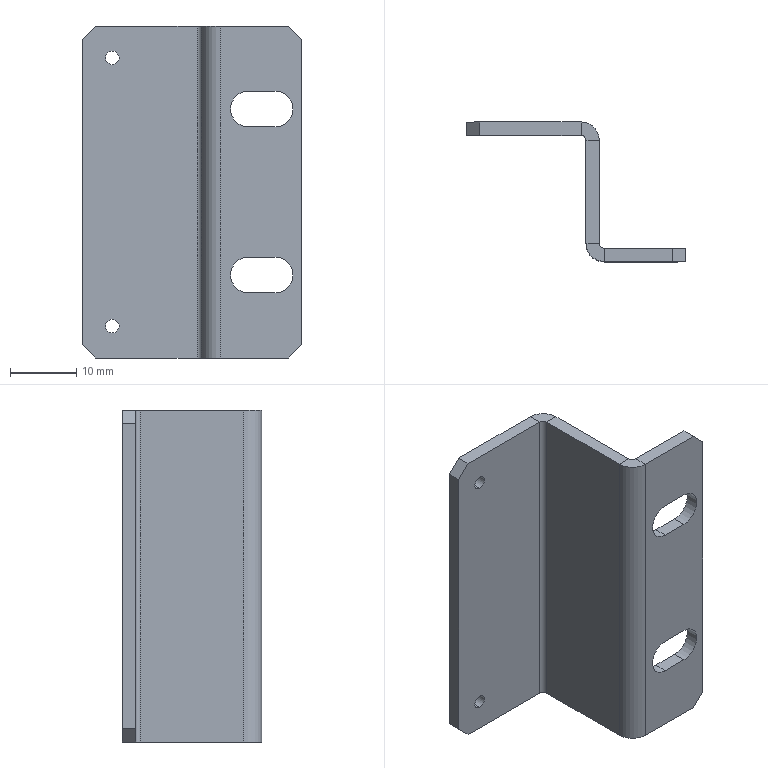Part | STEP file | 11-GYZB-JJ-00611 | 1 solid | 38 faces | box 33 x 21 x 50 mm | volume 4844 mm3 | plane 26 | cylinder 12 | commonest cylinder face diameters 2.05 x4 5.4 x4 1.473 x2 5.473 x2
STEP:
#1=CARTESIAN_POINT('',(-13.5,19.,-21.225));
#2=VERTEX_POINT('',#1);
#3=CARTESIAN_POINT('',(-13.5,19.,-19.175));
#4=VERTEX_POINT('',#3);
#5=CARTESIAN_POINT('',(-13.5,19.,-20.2));
#6=DIRECTION('',(0.,1.,0.));
#7=DIRECTION('',(-1.,0.,0.));
#8=AXIS2_PLACEMENT_3D('',#5,#6,#7);
#9=CIRCLE('',#8,1.025);
#10=EDGE_CURVE('',#2,#4,#9,.T.);
#11=ORIENTED_EDGE('',*,*,#10,.F.);
#12=CARTESIAN_POINT('',(-13.5,21.,-21.225));
#13=VERTEX_POINT('',#12);
#14=CARTESIAN_POINT('',(-13.5,21.,-21.225));
#15=DIRECTION('',(0.,1.,0.));
#16=VECTOR('',#15,1000.);
#17=LINE('',#14,#16);
#18=EDGE_CURVE('',#2,#13,#17,.T.);
#19=ORIENTED_EDGE('',*,*,#18,.T.);
#20=CARTESIAN_POINT('',(-13.5,21.,-19.175));
#21=VERTEX_POINT('',#20);
#22=CARTESIAN_POINT('',(-13.5,21.,-20.2));
#23=DIRECTION('',(0.,1.,0.));
#24=DIRECTION('',(0.,0.,1.));
#25=AXIS2_PLACEMENT_3D('',#22,#23,#24);
#26=CIRCLE('',#25,1.025);
#27=EDGE_CURVE('',#13,#21,#26,.T.);
#28=ORIENTED_EDGE('',*,*,#27,.T.);
#29=CARTESIAN_POINT('',(-13.5,21.,-19.175));
#30=DIRECTION('',(0.,1.,0.));
#31=VECTOR('',#30,1000.);
#32=LINE('',#29,#31);
#33=EDGE_CURVE('',#4,#21,#32,.T.);
#34=ORIENTED_EDGE('',*,*,#33,.F.);
#35=EDGE_LOOP('',(#11,#19,#28,#34));
#36=FACE_OUTER_BOUND('',#35,.T.);
#37=CARTESIAN_POINT('',(-13.5,21.,-20.2));
#38=DIRECTION('',(0.,1.,0.));
#39=DIRECTION('',(0.,0.,1.));
#40=AXIS2_PLACEMENT_3D('',#37,#38,#39);
#41=CYLINDRICAL_SURFACE('',#40,1.025);
#42=ADVANCED_FACE('',(#36),#41,.F.);
#43=CARTESIAN_POINT('',(-13.5,19.,19.175));
#44=VERTEX_POINT('',#43);
#45=CARTESIAN_POINT('',(-13.5,19.,21.225));
#46=VERTEX_POINT('',#45);
#47=CARTESIAN_POINT('',(-13.5,19.,20.2));
#48=DIRECTION('',(0.,1.,0.));
#49=DIRECTION('',(-1.,0.,0.));
#50=AXIS2_PLACEMENT_3D('',#47,#48,#49);
#51=CIRCLE('',#50,1.025);
#52=EDGE_CURVE('',#44,#46,#51,.T.);
#53=ORIENTED_EDGE('',*,*,#52,.F.);
#54=CARTESIAN_POINT('',(-13.5,21.,19.175));
#55=VERTEX_POINT('',#54);
#56=CARTESIAN_POINT('',(-13.5,21.,19.175));
#57=DIRECTION('',(0.,1.,0.));
#58=VECTOR('',#57,1000.);
#59=LINE('',#56,#58);
#60=EDGE_CURVE('',#44,#55,#59,.T.);
#61=ORIENTED_EDGE('',*,*,#60,.T.);
#62=CARTESIAN_POINT('',(-13.5,21.,21.225));
#63=VERTEX_POINT('',#62);
#64=CARTESIAN_POINT('',(-13.5,21.,20.2));
#65=DIRECTION('',(0.,1.,0.));
#66=DIRECTION('',(0.,0.,1.));
#67=AXIS2_PLACEMENT_3D('',#64,#65,#66);
#68=CIRCLE('',#67,1.025);
#69=EDGE_CURVE('',#55,#63,#68,.T.);
#70=ORIENTED_EDGE('',*,*,#69,.T.);
#71=CARTESIAN_POINT('',(-13.5,21.,21.225));
#72=DIRECTION('',(0.,1.,0.));
#73=VECTOR('',#72,1000.);
#74=LINE('',#71,#73);
#75=EDGE_CURVE('',#46,#63,#74,.T.);
#76=ORIENTED_EDGE('',*,*,#75,.F.);
#77=EDGE_LOOP('',(#53,#61,#70,#76));
#78=FACE_OUTER_BOUND('',#77,.T.);
#79=CARTESIAN_POINT('',(-13.5,21.,20.2));
#80=DIRECTION('',(0.,1.,0.));
#81=DIRECTION('',(0.,0.,1.));
#82=AXIS2_PLACEMENT_3D('',#79,#80,#81);
#83=CYLINDRICAL_SURFACE('',#82,1.025);
#84=ADVANCED_FACE('',(#78),#83,.F.);
#85=CARTESIAN_POINT('',(2.,18.263,-25.));
#86=VERTEX_POINT('',#85);
#87=CARTESIAN_POINT('',(2.,2.737,-25.));
#88=VERTEX_POINT('',#87);
#89=CARTESIAN_POINT('',(2.,0.,-25.));
#90=DIRECTION('',(0.,-1.,0.));
#91=VECTOR('',#90,1000.);
#92=LINE('',#89,#91);
#93=EDGE_CURVE('',#86,#88,#92,.T.);
#94=ORIENTED_EDGE('',*,*,#93,.F.);
#95=CARTESIAN_POINT('',(2.,18.263,25.));
#96=VERTEX_POINT('',#95);
#97=CARTESIAN_POINT('',(2.,18.263,-25.));
#98=DIRECTION('',(0.,0.,1.));
#99=VECTOR('',#98,1000.);
#100=LINE('',#97,#99);
#101=EDGE_CURVE('',#86,#96,#100,.T.);
#102=ORIENTED_EDGE('',*,*,#101,.T.);
#103=CARTESIAN_POINT('',(2.,2.737,25.));
#104=VERTEX_POINT('',#103);
#105=CARTESIAN_POINT('',(2.,0.,25.));
#106=DIRECTION('',(0.,-1.,0.));
#107=VECTOR('',#106,1000.);
#108=LINE('',#105,#107);
#109=EDGE_CURVE('',#96,#104,#108,.T.);
#110=ORIENTED_EDGE('',*,*,#109,.T.);
#111=CARTESIAN_POINT('',(2.,2.737,25.));
#112=DIRECTION('',(0.,0.,-1.));
#113=VECTOR('',#112,1000.);
#114=LINE('',#111,#113);
#115=EDGE_CURVE('',#104,#88,#114,.T.);
#116=ORIENTED_EDGE('',*,*,#115,.T.);
#117=EDGE_LOOP('',(#94,#102,#110,#116));
#118=FACE_OUTER_BOUND('',#117,.T.);
#119=CARTESIAN_POINT('',(2.,0.,25.));
#120=DIRECTION('',(1.,0.,0.));
#121=DIRECTION('',(0.,0.,-1.));
#122=AXIS2_PLACEMENT_3D('',#119,#120,#121);
#123=PLANE('',#122);
#124=ADVANCED_FACE('',(#118),#123,.T.);
#125=CARTESIAN_POINT('',(0.,18.263,-25.));
#126=VERTEX_POINT('',#125);
#127=CARTESIAN_POINT('',(0.,18.263,25.));
#128=VERTEX_POINT('',#127);
#129=CARTESIAN_POINT('',(0.,18.263,-25.));
#130=DIRECTION('',(0.,0.,1.));
#131=VECTOR('',#130,1000.);
#132=LINE('',#129,#131);
#133=EDGE_CURVE('',#126,#128,#132,.T.);
#134=ORIENTED_EDGE('',*,*,#133,.F.);
#135=CARTESIAN_POINT('',(0.,2.737,-25.));
#136=VERTEX_POINT('',#135);
#137=CARTESIAN_POINT('',(0.,0.,-25.));
#138=DIRECTION('',(0.,-1.,0.));
#139=VECTOR('',#138,1000.);
#140=LINE('',#137,#139);
#141=EDGE_CURVE('',#126,#136,#140,.T.);
#142=ORIENTED_EDGE('',*,*,#141,.T.);
#143=CARTESIAN_POINT('',(0.,2.737,25.));
#144=VERTEX_POINT('',#143);
#145=CARTESIAN_POINT('',(0.,2.737,25.));
#146=DIRECTION('',(0.,0.,-1.));
#147=VECTOR('',#146,1000.);
#148=LINE('',#145,#147);
#149=EDGE_CURVE('',#144,#136,#148,.T.);
#150=ORIENTED_EDGE('',*,*,#149,.F.);
#151=CARTESIAN_POINT('',(0.,0.,25.));
#152=DIRECTION('',(0.,-1.,0.));
#153=VECTOR('',#152,1000.);
#154=LINE('',#151,#153);
#155=EDGE_CURVE('',#128,#144,#154,.T.);
#156=ORIENTED_EDGE('',*,*,#155,.F.);
#157=EDGE_LOOP('',(#134,#142,#150,#156));
#158=FACE_OUTER_BOUND('',#157,.T.);
#159=CARTESIAN_POINT('',(0.,0.,25.));
#160=DIRECTION('',(1.,0.,0.));
#161=DIRECTION('',(0.,0.,-1.));
#162=AXIS2_PLACEMENT_3D('',#159,#160,#161);
#163=PLANE('',#162);
#164=ADVANCED_FACE('',(#158),#163,.F.);
#165=CARTESIAN_POINT('',(0.,18.263,-25.));
#166=DIRECTION('',(1.,0.,0.));
#167=VECTOR('',#166,1000.);
#168=LINE('',#165,#167);
#169=EDGE_CURVE('',#126,#86,#168,.T.);
#170=ORIENTED_EDGE('',*,*,#169,.T.);
#171=ORIENTED_EDGE('',*,*,#93,.T.);
#172=CARTESIAN_POINT('',(2.,2.737,-25.));
#173=DIRECTION('',(-1.,0.,0.));
#174=VECTOR('',#173,1000.);
#175=LINE('',#172,#174);
#176=EDGE_CURVE('',#88,#136,#175,.T.);
#177=ORIENTED_EDGE('',*,*,#176,.T.);
#178=ORIENTED_EDGE('',*,*,#141,.F.);
#179=EDGE_LOOP('',(#170,#171,#177,#178));
#180=FACE_OUTER_BOUND('',#179,.T.);
#181=CARTESIAN_POINT('',(2.737,2.737,-25.));
#182=DIRECTION('',(0.,0.,1.));
#183=DIRECTION('',(1.,0.,0.));
#184=AXIS2_PLACEMENT_3D('',#181,#182,#183);
#185=PLANE('',#184);
#186=ADVANCED_FACE('',(#180),#185,.F.);
#187=CARTESIAN_POINT('',(0.,2.737,25.));
#188=DIRECTION('',(1.,0.,0.));
#189=VECTOR('',#188,1000.);
#190=LINE('',#187,#189);
#191=EDGE_CURVE('',#144,#104,#190,.T.);
#192=ORIENTED_EDGE('',*,*,#191,.F.);
#193=CARTESIAN_POINT('',(2.737,0.,25.));
#194=VERTEX_POINT('',#193);
#195=CARTESIAN_POINT('',(2.737,2.737,25.));
#196=DIRECTION('',(0.,0.,1.));
#197=DIRECTION('',(-1.,0.,0.));
#198=AXIS2_PLACEMENT_3D('',#195,#196,#197);
#199=CIRCLE('',#198,2.737);
#200=EDGE_CURVE('',#144,#194,#199,.T.);
#201=ORIENTED_EDGE('',*,*,#200,.T.);
#202=CARTESIAN_POINT('',(2.737,2.,25.));
#203=VERTEX_POINT('',#202);
#204=CARTESIAN_POINT('',(2.737,2.,25.));
#205=DIRECTION('',(0.,-1.,0.));
#206=VECTOR('',#205,1000.);
#207=LINE('',#204,#206);
#208=EDGE_CURVE('',#203,#194,#207,.T.);
#209=ORIENTED_EDGE('',*,*,#208,.F.);
#210=CARTESIAN_POINT('',(2.737,2.737,25.));
#211=DIRECTION('',(0.,0.,1.));
#212=DIRECTION('',(1.,0.,0.));
#213=AXIS2_PLACEMENT_3D('',#210,#211,#212);
#214=CIRCLE('',#213,0.7366);
#215=EDGE_CURVE('',#104,#203,#214,.T.);
#216=ORIENTED_EDGE('',*,*,#215,.F.);
#217=EDGE_LOOP('',(#192,#201,#209,#216));
#218=FACE_OUTER_BOUND('',#217,.T.);
#219=CARTESIAN_POINT('',(0.,2.737,25.));
#220=DIRECTION('',(0.,0.,1.));
#221=DIRECTION('',(1.,0.,0.));
#222=AXIS2_PLACEMENT_3D('',#219,#220,#221);
#223=PLANE('',#222);
#224=ADVANCED_FACE('',(#218),#223,.T.);
#225=CARTESIAN_POINT('',(0.,18.263,25.));
#226=DIRECTION('',(1.,0.,0.));
#227=VECTOR('',#226,1000.);
#228=LINE('',#225,#227);
#229=EDGE_CURVE('',#128,#96,#228,.T.);
#230=ORIENTED_EDGE('',*,*,#229,.F.);
#231=ORIENTED_EDGE('',*,*,#155,.T.);
#232=ORIENTED_EDGE('',*,*,#191,.T.);
#233=ORIENTED_EDGE('',*,*,#109,.F.);
#234=EDGE_LOOP('',(#230,#231,#232,#233));
#235=FACE_OUTER_BOUND('',#234,.T.);
#236=CARTESIAN_POINT('',(2.737,2.,25.));
#237=DIRECTION('',(0.,0.,1.));
#238=DIRECTION('',(1.,0.,0.));
#239=AXIS2_PLACEMENT_3D('',#236,#237,#238);
#240=PLANE('',#239);
#241=ADVANCED_FACE('',(#235),#240,.T.);
#242=CARTESIAN_POINT('',(2.737,0.,-25.));
#243=VERTEX_POINT('',#242);
#244=CARTESIAN_POINT('',(2.737,2.,-25.));
#245=VERTEX_POINT('',#244);
#246=CARTESIAN_POINT('',(2.737,0.,-25.));
#247=DIRECTION('',(0.,1.,0.));
#248=VECTOR('',#247,1000.);
#249=LINE('',#246,#248);
#250=EDGE_CURVE('',#243,#245,#249,.T.);
#251=ORIENTED_EDGE('',*,*,#250,.F.);
#252=CARTESIAN_POINT('',(2.737,2.737,-25.));
#253=DIRECTION('',(0.,0.,1.));
#254=DIRECTION('',(-1.,0.,0.));
#255=AXIS2_PLACEMENT_3D('',#252,#253,#254);
#256=CIRCLE('',#255,2.737);
#257=EDGE_CURVE('',#136,#243,#256,.T.);
#258=ORIENTED_EDGE('',*,*,#257,.F.);
#259=ORIENTED_EDGE('',*,*,#176,.F.);
#260=CARTESIAN_POINT('',(2.737,2.737,-25.));
#261=DIRECTION('',(0.,0.,1.));
#262=DIRECTION('',(1.,0.,0.));
#263=AXIS2_PLACEMENT_3D('',#260,#261,#262);
#264=CIRCLE('',#263,0.7366);
#265=EDGE_CURVE('',#88,#245,#264,.T.);
#266=ORIENTED_EDGE('',*,*,#265,.T.);
#267=EDGE_LOOP('',(#251,#258,#259,#266));
#268=FACE_OUTER_BOUND('',#267,.T.);
#269=CARTESIAN_POINT('',(2.737,0.,-25.));
#270=DIRECTION('',(0.,0.,-1.));
#271=DIRECTION('',(-1.,0.,0.));
#272=AXIS2_PLACEMENT_3D('',#269,#270,#271);
#273=PLANE('',#272);
#274=ADVANCED_FACE('',(#268),#273,.T.);
#275=CARTESIAN_POINT('',(13.,2.,-25.));
#276=VERTEX_POINT('',#275);
#277=CARTESIAN_POINT('',(0.,2.,-25.));
#278=DIRECTION('',(1.,0.,0.));
#279=VECTOR('',#278,1000.);
#280=LINE('',#277,#279);
#281=EDGE_CURVE('',#245,#276,#280,.T.);
#282=ORIENTED_EDGE('',*,*,#281,.T.);
#283=CARTESIAN_POINT('',(13.,0.,-25.));
#284=VERTEX_POINT('',#283);
#285=CARTESIAN_POINT('',(13.,2.737,-25.));
#286=DIRECTION('',(0.,-1.,0.));
#287=VECTOR('',#286,1000.);
#288=LINE('',#285,#287);
#289=EDGE_CURVE('',#276,#284,#288,.T.);
#290=ORIENTED_EDGE('',*,*,#289,.T.);
#291=CARTESIAN_POINT('',(0.,0.,-25.));
#292=DIRECTION('',(1.,0.,0.));
#293=VECTOR('',#292,1000.);
#294=LINE('',#291,#293);
#295=EDGE_CURVE('',#243,#284,#294,.T.);
#296=ORIENTED_EDGE('',*,*,#295,.F.);
#297=ORIENTED_EDGE('',*,*,#250,.T.);
#298=EDGE_LOOP('',(#282,#290,#296,#297));
#299=FACE_OUTER_BOUND('',#298,.T.);
#300=CARTESIAN_POINT('',(2.,2.737,-25.));
#301=DIRECTION('',(0.,0.,-1.));
#302=DIRECTION('',(-1.,0.,0.));
#303=AXIS2_PLACEMENT_3D('',#300,#301,#302);
#304=PLANE('',#303);
#305=ADVANCED_FACE('',(#299),#304,.T.);
#306=CARTESIAN_POINT('',(11.,0.,-15.2));
#307=VERTEX_POINT('',#306);
#308=CARTESIAN_POINT('',(7.,0.,-15.2));
#309=VERTEX_POINT('',#308);
#310=CARTESIAN_POINT('',(7.,0.,-15.2));
#311=DIRECTION('',(-1.,0.,0.));
#312=VECTOR('',#311,1000.);
#313=LINE('',#310,#312);
#314=EDGE_CURVE('',#307,#309,#313,.T.);
#315=ORIENTED_EDGE('',*,*,#314,.T.);
#316=CARTESIAN_POINT('',(7.,0.,-9.8));
#317=VERTEX_POINT('',#316);
#318=CARTESIAN_POINT('',(7.,0.,-12.5));
#319=DIRECTION('',(0.,1.,0.));
#320=DIRECTION('',(0.,0.,-1.));
#321=AXIS2_PLACEMENT_3D('',#318,#319,#320);
#322=CIRCLE('',#321,2.7);
#323=EDGE_CURVE('',#309,#317,#322,.T.);
#324=ORIENTED_EDGE('',*,*,#323,.T.);
#325=CARTESIAN_POINT('',(11.,0.,-9.8));
#326=VERTEX_POINT('',#325);
#327=CARTESIAN_POINT('',(7.,0.,-9.8));
#328=DIRECTION('',(1.,0.,0.));
#329=VECTOR('',#328,1000.);
#330=LINE('',#327,#329);
#331=EDGE_CURVE('',#317,#326,#330,.T.);
#332=ORIENTED_EDGE('',*,*,#331,.T.);
#333=CARTESIAN_POINT('',(11.,0.,-12.5));
#334=DIRECTION('',(0.,1.,0.));
#335=DIRECTION('',(0.,0.,-1.));
#336=AXIS2_PLACEMENT_3D('',#333,#334,#335);
#337=CIRCLE('',#336,2.7);
#338=EDGE_CURVE('',#326,#307,#337,.T.);
#339=ORIENTED_EDGE('',*,*,#338,.T.);
#340=EDGE_LOOP('',(#315,#324,#332,#339));
#341=FACE_BOUND('',#340,.T.);
#342=CARTESIAN_POINT('',(11.,0.,9.8));
#343=VERTEX_POINT('',#342);
#344=CARTESIAN_POINT('',(7.,0.,9.8));
#345=VERTEX_POINT('',#344);
#346=CARTESIAN_POINT('',(7.,0.,9.8));
#347=DIRECTION('',(-1.,0.,0.));
#348=VECTOR('',#347,1000.);
#349=LINE('',#346,#348);
#350=EDGE_CURVE('',#343,#345,#349,.T.);
#351=ORIENTED_EDGE('',*,*,#350,.T.);
#352=CARTESIAN_POINT('',(7.,0.,15.2));
#353=VERTEX_POINT('',#352);
#354=CARTESIAN_POINT('',(7.,0.,12.5));
#355=DIRECTION('',(0.,1.,0.));
#356=DIRECTION('',(0.,0.,1.));
#357=AXIS2_PLACEMENT_3D('',#354,#355,#356);
#358=CIRCLE('',#357,2.7);
#359=EDGE_CURVE('',#345,#353,#358,.T.);
#360=ORIENTED_EDGE('',*,*,#359,.T.);
#361=CARTESIAN_POINT('',(11.,0.,15.2));
#362=VERTEX_POINT('',#361);
#363=CARTESIAN_POINT('',(7.,0.,15.2));
#364=DIRECTION('',(1.,0.,0.));
#365=VECTOR('',#364,1000.);
#366=LINE('',#363,#365);
#367=EDGE_CURVE('',#353,#362,#366,.T.);
#368=ORIENTED_EDGE('',*,*,#367,.T.);
#369=CARTESIAN_POINT('',(11.,0.,12.5));
#370=DIRECTION('',(0.,1.,0.));
#371=DIRECTION('',(0.,0.,1.));
#372=AXIS2_PLACEMENT_3D('',#369,#370,#371);
#373=CIRCLE('',#372,2.7);
#374=EDGE_CURVE('',#362,#343,#373,.T.);
#375=ORIENTED_EDGE('',*,*,#374,.T.);
#376=EDGE_LOOP('',(#351,#360,#368,#375));
#377=FACE_BOUND('',#376,.T.);
#378=CARTESIAN_POINT('',(15.,0.,23.));
#379=VERTEX_POINT('',#378);
#380=CARTESIAN_POINT('',(15.,0.,-23.));
#381=VERTEX_POINT('',#380);
#382=CARTESIAN_POINT('',(15.,0.,25.));
#383=DIRECTION('',(0.,0.,-1.));
#384=VECTOR('',#383,1000.);
#385=LINE('',#382,#384);
#386=EDGE_CURVE('',#379,#381,#385,.T.);
#387=ORIENTED_EDGE('',*,*,#386,.F.);
#388=CARTESIAN_POINT('',(13.,0.,25.));
#389=VERTEX_POINT('',#388);
#390=CARTESIAN_POINT('',(15.,0.,23.));
#391=DIRECTION('',(-0.7071,0.,0.7071));
#392=VECTOR('',#391,1000.);
#393=LINE('',#390,#392);
#394=EDGE_CURVE('',#379,#389,#393,.T.);
#395=ORIENTED_EDGE('',*,*,#394,.T.);
#396=CARTESIAN_POINT('',(0.,0.,25.));
#397=DIRECTION('',(1.,0.,0.));
#398=VECTOR('',#397,1000.);
#399=LINE('',#396,#398);
#400=EDGE_CURVE('',#194,#389,#399,.T.);
#401=ORIENTED_EDGE('',*,*,#400,.F.);
#402=CARTESIAN_POINT('',(2.737,0.,25.));
#403=DIRECTION('',(0.,0.,-1.));
#404=VECTOR('',#403,1000.);
#405=LINE('',#402,#404);
#406=EDGE_CURVE('',#194,#243,#405,.T.);
#407=ORIENTED_EDGE('',*,*,#406,.T.);
#408=ORIENTED_EDGE('',*,*,#295,.T.);
#409=CARTESIAN_POINT('',(13.,0.,-25.));
#410=DIRECTION('',(0.7071,0.,0.7071));
#411=VECTOR('',#410,1000.);
#412=LINE('',#409,#411);
#413=EDGE_CURVE('',#284,#381,#412,.T.);
#414=ORIENTED_EDGE('',*,*,#413,.T.);
#415=EDGE_LOOP('',(#387,#395,#401,#407,#408,#414));
#416=FACE_OUTER_BOUND('',#415,.T.);
#417=CARTESIAN_POINT('',(0.,0.,25.));
#418=DIRECTION('',(0.,1.,0.));
#419=DIRECTION('',(0.,0.,1.));
#420=AXIS2_PLACEMENT_3D('',#417,#418,#419);
#421=PLANE('',#420);
#422=ADVANCED_FACE('',(#341,#377,#416),#421,.F.);
#423=CARTESIAN_POINT('',(15.,2.,23.));
#424=VERTEX_POINT('',#423);
#425=CARTESIAN_POINT('',(15.,2.,-23.));
#426=VERTEX_POINT('',#425);
#427=CARTESIAN_POINT('',(15.,2.,25.));
#428=DIRECTION('',(0.,0.,-1.));
#429=VECTOR('',#428,1000.);
#430=LINE('',#427,#429);
#431=EDGE_CURVE('',#424,#426,#430,.T.);
#432=ORIENTED_EDGE('',*,*,#431,.F.);
#433=CARTESIAN_POINT('',(15.,2.,23.));
#434=DIRECTION('',(0.,-1.,0.));
#435=VECTOR('',#434,1000.);
#436=LINE('',#433,#435);
#437=EDGE_CURVE('',#424,#379,#436,.T.);
#438=ORIENTED_EDGE('',*,*,#437,.T.);
#439=ORIENTED_EDGE('',*,*,#386,.T.);
#440=CARTESIAN_POINT('',(15.,2.,-23.));
#441=DIRECTION('',(0.,1.,0.));
#442=VECTOR('',#441,1000.);
#443=LINE('',#440,#442);
#444=EDGE_CURVE('',#381,#426,#443,.T.);
#445=ORIENTED_EDGE('',*,*,#444,.T.);
#446=EDGE_LOOP('',(#432,#438,#439,#445));
#447=FACE_OUTER_BOUND('',#446,.T.);
#448=CARTESIAN_POINT('',(15.,2.,25.));
#449=DIRECTION('',(1.,0.,0.));
#450=DIRECTION('',(0.,0.,-1.));
#451=AXIS2_PLACEMENT_3D('',#448,#449,#450);
#452=PLANE('',#451);
#453=ADVANCED_FACE('',(#447),#452,.T.);
#454=CARTESIAN_POINT('',(7.,2.,-15.2));
#455=VERTEX_POINT('',#454);
#456=CARTESIAN_POINT('',(7.,2.,-9.8));
#457=VERTEX_POINT('',#456);
#458=CARTESIAN_POINT('',(7.,2.,-12.5));
#459=DIRECTION('',(0.,1.,0.));
#460=DIRECTION('',(0.,0.,-1.));
#461=AXIS2_PLACEMENT_3D('',#458,#459,#460);
#462=CIRCLE('',#461,2.7);
#463=EDGE_CURVE('',#455,#457,#462,.T.);
#464=ORIENTED_EDGE('',*,*,#463,.F.);
#465=CARTESIAN_POINT('',(11.,2.,-15.2));
#466=VERTEX_POINT('',#465);
#467=CARTESIAN_POINT('',(7.,2.,-15.2));
#468=DIRECTION('',(-1.,0.,0.));
#469=VECTOR('',#468,1000.);
#470=LINE('',#467,#469);
#471=EDGE_CURVE('',#466,#455,#470,.T.);
#472=ORIENTED_EDGE('',*,*,#471,.F.);
#473=CARTESIAN_POINT('',(11.,2.,-9.8));
#474=VERTEX_POINT('',#473);
#475=CARTESIAN_POINT('',(11.,2.,-12.5));
#476=DIRECTION('',(0.,1.,0.));
#477=DIRECTION('',(0.,0.,-1.));
#478=AXIS2_PLACEMENT_3D('',#475,#476,#477);
#479=CIRCLE('',#478,2.7);
#480=EDGE_CURVE('',#474,#466,#479,.T.);
#481=ORIENTED_EDGE('',*,*,#480,.F.);
#482=CARTESIAN_POINT('',(7.,2.,-9.8));
#483=DIRECTION('',(1.,0.,0.));
#484=VECTOR('',#483,1000.);
#485=LINE('',#482,#484);
#486=EDGE_CURVE('',#457,#474,#485,.T.);
#487=ORIENTED_EDGE('',*,*,#486,.F.);
#488=EDGE_LOOP('',(#464,#472,#481,#487));
#489=FACE_BOUND('',#488,.T.);
#490=CARTESIAN_POINT('',(7.,2.,9.8));
#491=VERTEX_POINT('',#490);
#492=CARTESIAN_POINT('',(7.,2.,15.2));
#493=VERTEX_POINT('',#492);
#494=CARTESIAN_POINT('',(7.,2.,12.5));
#495=DIRECTION('',(0.,1.,0.));
#496=DIRECTION('',(0.,0.,1.));
#497=AXIS2_PLACEMENT_3D('',#494,#495,#496);
#498=CIRCLE('',#497,2.7);
#499=EDGE_CURVE('',#491,#493,#498,.T.);
#500=ORIENTED_EDGE('',*,*,#499,.F.);
#501=CARTESIAN_POINT('',(11.,2.,9.8));
#502=VERTEX_POINT('',#501);
#503=CARTESIAN_POINT('',(7.,2.,9.8));
#504=DIRECTION('',(-1.,0.,0.));
#505=VECTOR('',#504,1000.);
#506=LINE('',#503,#505);
#507=EDGE_CURVE('',#502,#491,#506,.T.);
#508=ORIENTED_EDGE('',*,*,#507,.F.);
#509=CARTESIAN_POINT('',(11.,2.,15.2));
#510=VERTEX_POINT('',#509);
#511=CARTESIAN_POINT('',(11.,2.,12.5));
#512=DIRECTION('',(0.,1.,0.));
#513=DIRECTION('',(0.,0.,1.));
#514=AXIS2_PLACEMENT_3D('',#511,#512,#513);
#515=CIRCLE('',#514,2.7);
#516=EDGE_CURVE('',#510,#502,#515,.T.);
#517=ORIENTED_EDGE('',*,*,#516,.F.);
#518=CARTESIAN_POINT('',(7.,2.,15.2));
#519=DIRECTION('',(1.,0.,0.));
#520=VECTOR('',#519,1000.);
#521=LINE('',#518,#520);
#522=EDGE_CURVE('',#493,#510,#521,.T.);
#523=ORIENTED_EDGE('',*,*,#522,.F.);
#524=EDGE_LOOP('',(#500,#508,#517,#523));
#525=FACE_BOUND('',#524,.T.);
#526=CARTESIAN_POINT('',(13.,2.,25.));
#527=VERTEX_POINT('',#526);
#528=CARTESIAN_POINT('',(0.,2.,25.));
#529=DIRECTION('',(1.,0.,0.));
#530=VECTOR('',#529,1000.);
#531=LINE('',#528,#530);
#532=EDGE_CURVE('',#203,#527,#531,.T.);
#533=ORIENTED_EDGE('',*,*,#532,.T.);
#534=CARTESIAN_POINT('',(6.5,2.,31.5));
#535=DIRECTION('',(0.7071,0.,-0.7071));
#536=VECTOR('',#535,1000.);
#537=LINE('',#534,#536);
#538=EDGE_CURVE('',#527,#424,#537,.T.);
#539=ORIENTED_EDGE('',*,*,#538,.T.);
#540=ORIENTED_EDGE('',*,*,#431,.T.);
#541=CARTESIAN_POINT('',(31.5,2.,-6.5));
#542=DIRECTION('',(-0.7071,0.,-0.7071));
#543=VECTOR('',#542,1000.);
#544=LINE('',#541,#543);
#545=EDGE_CURVE('',#426,#276,#544,.T.);
#546=ORIENTED_EDGE('',*,*,#545,.T.);
#547=ORIENTED_EDGE('',*,*,#281,.F.);
#548=CARTESIAN_POINT('',(2.737,2.,25.));
#549=DIRECTION('',(0.,0.,-1.));
#550=VECTOR('',#549,1000.);
#551=LINE('',#548,#550);
#552=EDGE_CURVE('',#203,#245,#551,.T.);
#553=ORIENTED_EDGE('',*,*,#552,.F.);
#554=EDGE_LOOP('',(#533,#539,#540,#546,#547,#553));
#555=FACE_OUTER_BOUND('',#554,.T.);
#556=CARTESIAN_POINT('',(0.,2.,25.));
#557=DIRECTION('',(0.,1.,0.));
#558=DIRECTION('',(0.,0.,1.));
#559=AXIS2_PLACEMENT_3D('',#556,#557,#558);
#560=PLANE('',#559);
#561=ADVANCED_FACE('',(#489,#525,#555),#560,.T.);
#562=ORIENTED_EDGE('',*,*,#265,.F.);
#563=ORIENTED_EDGE('',*,*,#115,.F.);
#564=ORIENTED_EDGE('',*,*,#215,.T.);
#565=ORIENTED_EDGE('',*,*,#552,.T.);
#566=EDGE_LOOP('',(#562,#563,#564,#565));
#567=FACE_OUTER_BOUND('',#566,.T.);
#568=CARTESIAN_POINT('',(2.737,2.737,25.));
#569=DIRECTION('',(0.,0.,-1.));
#570=DIRECTION('',(-1.,0.,0.));
#571=AXIS2_PLACEMENT_3D('',#568,#569,#570);
#572=CYLINDRICAL_SURFACE('',#571,0.7366);
#573=ADVANCED_FACE('',(#567),#572,.F.);
#574=ORIENTED_EDGE('',*,*,#257,.T.);
#575=ORIENTED_EDGE('',*,*,#406,.F.);
#576=ORIENTED_EDGE('',*,*,#200,.F.);
#577=ORIENTED_EDGE('',*,*,#149,.T.);
#578=EDGE_LOOP('',(#574,#575,#576,#577));
#579=FACE_OUTER_BOUND('',#578,.T.);
#580=CARTESIAN_POINT('',(2.737,2.737,25.));
#581=DIRECTION('',(0.,0.,-1.));
#582=DIRECTION('',(-1.,0.,0.));
#583=AXIS2_PLACEMENT_3D('',#580,#581,#582);
#584=CYLINDRICAL_SURFACE('',#583,2.737);
#585=ADVANCED_FACE('',(#579),#584,.T.);
#586=ORIENTED_EDGE('',*,*,#400,.T.);
#587=CARTESIAN_POINT('',(13.,2.737,25.));
#588=DIRECTION('',(0.,1.,0.));
#589=VECTOR('',#588,1000.);
#590=LINE('',#587,#589);
#591=EDGE_CURVE('',#389,#527,#590,.T.);
#592=ORIENTED_EDGE('',*,*,#591,.T.);
#593=ORIENTED_EDGE('',*,*,#532,.F.);
#594=ORIENTED_EDGE('',*,*,#208,.T.);
#595=EDGE_LOOP('',(#586,#592,#593,#594));
#596=FACE_OUTER_BOUND('',#595,.T.);
#597=CARTESIAN_POINT('',(2.737,2.737,25.));
#598=DIRECTION('',(0.,0.,1.));
#599=DIRECTION('',(1.,0.,0.));
#600=AXIS2_PLACEMENT_3D('',#597,#598,#599);
#601=PLANE('',#600);
#602=ADVANCED_FACE('',(#596),#601,.T.);
#603=ORIENTED_EDGE('',*,*,#499,.T.);
#604=CARTESIAN_POINT('',(7.,0.,15.2));
#605=DIRECTION('',(0.,1.,0.));
#606=VECTOR('',#605,1000.);
#607=LINE('',#604,#606);
#608=EDGE_CURVE('',#353,#493,#607,.T.);
#609=ORIENTED_EDGE('',*,*,#608,.F.);
#610=ORIENTED_EDGE('',*,*,#359,.F.);
#611=CARTESIAN_POINT('',(7.,0.,9.8));
#612=DIRECTION('',(0.,1.,0.));
#613=VECTOR('',#612,1000.);
#614=LINE('',#611,#613);
#615=EDGE_CURVE('',#345,#491,#614,.T.);
#616=ORIENTED_EDGE('',*,*,#615,.T.);
#617=EDGE_LOOP('',(#603,#609,#610,#616));
#618=FACE_OUTER_BOUND('',#617,.T.);
#619=CARTESIAN_POINT('',(7.,0.,12.5));
#620=DIRECTION('',(0.,1.,0.));
#621=DIRECTION('',(0.,0.,1.));
#622=AXIS2_PLACEMENT_3D('',#619,#620,#621);
#623=CYLINDRICAL_SURFACE('',#622,2.7);
#624=ADVANCED_FACE('',(#618),#623,.F.);
#625=ORIENTED_EDGE('',*,*,#507,.T.);
#626=ORIENTED_EDGE('',*,*,#615,.F.);
#627=ORIENTED_EDGE('',*,*,#350,.F.);
#628=CARTESIAN_POINT('',(11.,0.,9.8));
#629=DIRECTION('',(0.,1.,0.));
#630=VECTOR('',#629,1000.);
#631=LINE('',#628,#630);
#632=EDGE_CURVE('',#343,#502,#631,.T.);
#633=ORIENTED_EDGE('',*,*,#632,.T.);
#634=EDGE_LOOP('',(#625,#626,#627,#633));
#635=FACE_OUTER_BOUND('',#634,.T.);
#636=CARTESIAN_POINT('',(7.,0.,9.8));
#637=DIRECTION('',(0.,0.,-1.));
#638=DIRECTION('',(-1.,0.,0.));
#639=AXIS2_PLACEMENT_3D('',#636,#637,#638);
#640=PLANE('',#639);
#641=ADVANCED_FACE('',(#635),#640,.F.);
#642=ORIENTED_EDGE('',*,*,#516,.T.);
#643=ORIENTED_EDGE('',*,*,#632,.F.);
#644=ORIENTED_EDGE('',*,*,#374,.F.);
#645=CARTESIAN_POINT('',(11.,0.,15.2));
#646=DIRECTION('',(0.,1.,0.));
#647=VECTOR('',#646,1000.);
#648=LINE('',#645,#647);
#649=EDGE_CURVE('',#362,#510,#648,.T.);
#650=ORIENTED_EDGE('',*,*,#649,.T.);
#651=EDGE_LOOP('',(#642,#643,#644,#650));
#652=FACE_OUTER_BOUND('',#651,.T.);
#653=CARTESIAN_POINT('',(11.,0.,12.5));
#654=DIRECTION('',(0.,1.,0.));
#655=DIRECTION('',(0.,0.,1.));
#656=AXIS2_PLACEMENT_3D('',#653,#654,#655);
#657=CYLINDRICAL_SURFACE('',#656,2.7);
#658=ADVANCED_FACE('',(#652),#657,.F.);
#659=ORIENTED_EDGE('',*,*,#522,.T.);
#660=ORIENTED_EDGE('',*,*,#649,.F.);
#661=ORIENTED_EDGE('',*,*,#367,.F.);
#662=ORIENTED_EDGE('',*,*,#608,.T.);
#663=EDGE_LOOP('',(#659,#660,#661,#662));
#664=FACE_OUTER_BOUND('',#663,.T.);
#665=CARTESIAN_POINT('',(7.,0.,15.2));
#666=DIRECTION('',(0.,0.,1.));
#667=DIRECTION('',(1.,0.,0.));
#668=AXIS2_PLACEMENT_3D('',#665,#666,#667);
#669=PLANE('',#668);
#670=ADVANCED_FACE('',(#664),#669,.F.);
#671=ORIENTED_EDGE('',*,*,#463,.T.);
#672=CARTESIAN_POINT('',(7.,0.,-9.8));
#673=DIRECTION('',(0.,1.,0.));
#674=VECTOR('',#673,1000.);
#675=LINE('',#672,#674);
#676=EDGE_CURVE('',#317,#457,#675,.T.);
#677=ORIENTED_EDGE('',*,*,#676,.F.);
#678=ORIENTED_EDGE('',*,*,#323,.F.);
#679=CARTESIAN_POINT('',(7.,0.,-15.2));
#680=DIRECTION('',(0.,1.,0.));
#681=VECTOR('',#680,1000.);
#682=LINE('',#679,#681);
#683=EDGE_CURVE('',#309,#455,#682,.T.);
#684=ORIENTED_EDGE('',*,*,#683,.T.);
#685=EDGE_LOOP('',(#671,#677,#678,#684));
#686=FACE_OUTER_BOUND('',#685,.T.);
#687=CARTESIAN_POINT('',(7.,0.,-12.5));
#688=DIRECTION('',(0.,1.,0.));
#689=DIRECTION('',(0.,0.,1.));
#690=AXIS2_PLACEMENT_3D('',#687,#688,#689);
#691=CYLINDRICAL_SURFACE('',#690,2.7);
#692=ADVANCED_FACE('',(#686),#691,.F.);
#693=ORIENTED_EDGE('',*,*,#471,.T.);
#694=ORIENTED_EDGE('',*,*,#683,.F.);
#695=ORIENTED_EDGE('',*,*,#314,.F.);
#696=CARTESIAN_POINT('',(11.,0.,-15.2));
#697=DIRECTION('',(0.,1.,0.));
#698=VECTOR('',#697,1000.);
#699=LINE('',#696,#698);
#700=EDGE_CURVE('',#307,#466,#699,.T.);
#701=ORIENTED_EDGE('',*,*,#700,.T.);
#702=EDGE_LOOP('',(#693,#694,#695,#701));
#703=FACE_OUTER_BOUND('',#702,.T.);
#704=CARTESIAN_POINT('',(7.,0.,-15.2));
#705=DIRECTION('',(0.,0.,-1.));
#706=DIRECTION('',(-1.,0.,0.));
#707=AXIS2_PLACEMENT_3D('',#704,#705,#706);
#708=PLANE('',#707);
#709=ADVANCED_FACE('',(#703),#708,.F.);
#710=ORIENTED_EDGE('',*,*,#480,.T.);
#711=ORIENTED_EDGE('',*,*,#700,.F.);
#712=ORIENTED_EDGE('',*,*,#338,.F.);
#713=CARTESIAN_POINT('',(11.,0.,-9.8));
#714=DIRECTION('',(0.,1.,0.));
#715=VECTOR('',#714,1000.);
#716=LINE('',#713,#715);
#717=EDGE_CURVE('',#326,#474,#716,.T.);
#718=ORIENTED_EDGE('',*,*,#717,.T.);
#719=EDGE_LOOP('',(#710,#711,#712,#718));
#720=FACE_OUTER_BOUND('',#719,.T.);
#721=CARTESIAN_POINT('',(11.,0.,-12.5));
#722=DIRECTION('',(0.,1.,0.));
#723=DIRECTION('',(0.,0.,1.));
#724=AXIS2_PLACEMENT_3D('',#721,#722,#723);
#725=CYLINDRICAL_SURFACE('',#724,2.7);
#726=ADVANCED_FACE('',(#720),#725,.F.);
#727=ORIENTED_EDGE('',*,*,#486,.T.);
#728=ORIENTED_EDGE('',*,*,#717,.F.);
#729=ORIENTED_EDGE('',*,*,#331,.F.);
#730=ORIENTED_EDGE('',*,*,#676,.T.);
#731=EDGE_LOOP('',(#727,#728,#729,#730));
#732=FACE_OUTER_BOUND('',#731,.T.);
#733=CARTESIAN_POINT('',(7.,0.,-9.8));
#734=DIRECTION('',(0.,0.,1.));
#735=DIRECTION('',(1.,0.,0.));
#736=AXIS2_PLACEMENT_3D('',#733,#734,#735);
#737=PLANE('',#736);
#738=ADVANCED_FACE('',(#732),#737,.F.);
#739=CARTESIAN_POINT('',(-0.7366,19.,25.));
#740=VERTEX_POINT('',#739);
#741=CARTESIAN_POINT('',(-0.7366,21.,25.));
#742=VERTEX_POINT('',#741);
#743=CARTESIAN_POINT('',(-0.7366,21.,25.));
#744=DIRECTION('',(0.,1.,0.));
#745=VECTOR('',#744,1000.);
#746=LINE('',#743,#745);
#747=EDGE_CURVE('',#740,#742,#746,.T.);
#748=ORIENTED_EDGE('',*,*,#747,.F.);
#749=CARTESIAN_POINT('',(-0.7366,18.263,25.));
#750=DIRECTION('',(0.,0.,1.));
#751=DIRECTION('',(-1.,0.,0.));
#752=AXIS2_PLACEMENT_3D('',#749,#750,#751);
#753=CIRCLE('',#752,0.7366);
#754=EDGE_CURVE('',#128,#740,#753,.T.);
#755=ORIENTED_EDGE('',*,*,#754,.F.);
#756=ORIENTED_EDGE('',*,*,#229,.T.);
#757=CARTESIAN_POINT('',(-0.7366,18.263,25.));
#758=DIRECTION('',(0.,0.,1.));
#759=DIRECTION('',(-1.,0.,0.));
#760=AXIS2_PLACEMENT_3D('',#757,#758,#759);
#761=CIRCLE('',#760,2.737);
#762=EDGE_CURVE('',#96,#742,#761,.T.);
#763=ORIENTED_EDGE('',*,*,#762,.T.);
#764=EDGE_LOOP('',(#748,#755,#756,#763));
#765=FACE_OUTER_BOUND('',#764,.T.);
#766=CARTESIAN_POINT('',(-0.7366,18.263,25.));
#767=DIRECTION('',(0.,0.,1.));
#768=DIRECTION('',(1.,0.,0.));
#769=AXIS2_PLACEMENT_3D('',#766,#767,#768);
#770=PLANE('',#769);
#771=ADVANCED_FACE('',(#765),#770,.T.);
#772=CARTESIAN_POINT('',(-0.7366,19.,-25.));
#773=VERTEX_POINT('',#772);
#774=CARTESIAN_POINT('',(-0.7366,18.263,-25.));
#775=DIRECTION('',(0.,0.,-1.));
#776=DIRECTION('',(-1.,0.,0.));
#777=AXIS2_PLACEMENT_3D('',#774,#775,#776);
#778=CIRCLE('',#777,0.7366);
#779=EDGE_CURVE('',#773,#126,#778,.T.);
#780=ORIENTED_EDGE('',*,*,#779,.F.);
#781=CARTESIAN_POINT('',(-0.7366,21.,-25.));
#782=VERTEX_POINT('',#781);
#783=CARTESIAN_POINT('',(-0.7366,19.,-25.));
#784=DIRECTION('',(0.,1.,0.));
#785=VECTOR('',#784,1000.);
#786=LINE('',#783,#785);
#787=EDGE_CURVE('',#773,#782,#786,.T.);
#788=ORIENTED_EDGE('',*,*,#787,.T.);
#789=CARTESIAN_POINT('',(-0.7366,18.263,-25.));
#790=DIRECTION('',(0.,0.,-1.));
#791=DIRECTION('',(-1.,0.,0.));
#792=AXIS2_PLACEMENT_3D('',#789,#790,#791);
#793=CIRCLE('',#792,2.737);
#794=EDGE_CURVE('',#782,#86,#793,.T.);
#795=ORIENTED_EDGE('',*,*,#794,.T.);
#796=ORIENTED_EDGE('',*,*,#169,.F.);
#797=EDGE_LOOP('',(#780,#788,#795,#796));
#798=FACE_OUTER_BOUND('',#797,.T.);
#799=CARTESIAN_POINT('',(-0.7366,18.263,-25.));
#800=DIRECTION('',(0.,0.,1.));
#801=DIRECTION('',(1.,0.,0.));
#802=AXIS2_PLACEMENT_3D('',#799,#800,#801);
#803=PLANE('',#802);
#804=ADVANCED_FACE('',(#798),#803,.F.);
#805=ORIENTED_EDGE('',*,*,#101,.F.);
#806=ORIENTED_EDGE('',*,*,#794,.F.);
#807=CARTESIAN_POINT('',(-0.7366,21.,0.));
#808=DIRECTION('',(0.,0.,-1.));
#809=VECTOR('',#808,1000.);
#810=LINE('',#807,#809);
#811=EDGE_CURVE('',#742,#782,#810,.T.);
#812=ORIENTED_EDGE('',*,*,#811,.F.);
#813=ORIENTED_EDGE('',*,*,#762,.F.);
#814=EDGE_LOOP('',(#805,#806,#812,#813));
#815=FACE_OUTER_BOUND('',#814,.T.);
#816=CARTESIAN_POINT('',(-0.7366,18.263,-25.));
#817=DIRECTION('',(0.,0.,-1.));
#818=DIRECTION('',(0.,1.,0.));
#819=AXIS2_PLACEMENT_3D('',#816,#817,#818);
#820=CYLINDRICAL_SURFACE('',#819,2.737);
#821=ADVANCED_FACE('',(#815),#820,.T.);
#822=ORIENTED_EDGE('',*,*,#133,.T.);
#823=ORIENTED_EDGE('',*,*,#754,.T.);
#824=CARTESIAN_POINT('',(-0.7366,19.,25.));
#825=DIRECTION('',(0.,0.,-1.));
#826=VECTOR('',#825,1000.);
#827=LINE('',#824,#826);
#828=EDGE_CURVE('',#740,#773,#827,.T.);
#829=ORIENTED_EDGE('',*,*,#828,.T.);
#830=ORIENTED_EDGE('',*,*,#779,.T.);
#831=EDGE_LOOP('',(#822,#823,#829,#830));
#832=FACE_OUTER_BOUND('',#831,.T.);
#833=CARTESIAN_POINT('',(-0.7366,18.263,-25.));
#834=DIRECTION('',(0.,0.,-1.));
#835=DIRECTION('',(0.,1.,0.));
#836=AXIS2_PLACEMENT_3D('',#833,#834,#835);
#837=CYLINDRICAL_SURFACE('',#836,0.7366);
#838=ADVANCED_FACE('',(#832),#837,.F.);
#839=CARTESIAN_POINT('',(-16.,19.,-25.));
#840=VERTEX_POINT('',#839);
#841=CARTESIAN_POINT('',(0.,19.,-25.));
#842=DIRECTION('',(1.,0.,0.));
#843=VECTOR('',#842,1000.);
#844=LINE('',#841,#843);
#845=EDGE_CURVE('',#840,#773,#844,.T.);
#846=ORIENTED_EDGE('',*,*,#845,.F.);
#847=CARTESIAN_POINT('',(-16.,21.,-25.));
#848=VERTEX_POINT('',#847);
#849=CARTESIAN_POINT('',(-16.,21.,-25.));
#850=DIRECTION('',(0.,1.,0.));
#851=VECTOR('',#850,1000.);
#852=LINE('',#849,#851);
#853=EDGE_CURVE('',#840,#848,#852,.T.);
#854=ORIENTED_EDGE('',*,*,#853,.T.);
#855=CARTESIAN_POINT('',(0.,21.,-25.));
#856=DIRECTION('',(1.,0.,0.));
#857=VECTOR('',#856,1000.);
#858=LINE('',#855,#857);
#859=EDGE_CURVE('',#848,#782,#858,.T.);
#860=ORIENTED_EDGE('',*,*,#859,.T.);
#861=ORIENTED_EDGE('',*,*,#787,.F.);
#862=EDGE_LOOP('',(#846,#854,#860,#861));
#863=FACE_OUTER_BOUND('',#862,.T.);
#864=CARTESIAN_POINT('',(0.,21.,-25.));
#865=DIRECTION('',(0.,0.,-1.));
#866=DIRECTION('',(-1.,0.,0.));
#867=AXIS2_PLACEMENT_3D('',#864,#865,#866);
#868=PLANE('',#867);
#869=ADVANCED_FACE('',(#863),#868,.T.);
#870=CARTESIAN_POINT('',(-16.,21.,25.));
#871=VERTEX_POINT('',#870);
#872=CARTESIAN_POINT('',(-18.,21.,25.));
#873=DIRECTION('',(-1.,0.,0.));
#874=VECTOR('',#873,1000.);
#875=LINE('',#872,#874);
#876=EDGE_CURVE('',#742,#871,#875,.T.);
#877=ORIENTED_EDGE('',*,*,#876,.T.);
#878=CARTESIAN_POINT('',(-16.,19.,25.));
#879=VERTEX_POINT('',#878);
#880=CARTESIAN_POINT('',(-16.,21.,25.));
#881=DIRECTION('',(0.,-1.,0.));
#882=VECTOR('',#881,1000.);
#883=LINE('',#880,#882);
#884=EDGE_CURVE('',#871,#879,#883,.T.);
#885=ORIENTED_EDGE('',*,*,#884,.T.);
#886=CARTESIAN_POINT('',(0.,19.,25.));
#887=DIRECTION('',(-1.,0.,0.));
#888=VECTOR('',#887,1000.);
#889=LINE('',#886,#888);
#890=EDGE_CURVE('',#740,#879,#889,.T.);
#891=ORIENTED_EDGE('',*,*,#890,.F.);
#892=ORIENTED_EDGE('',*,*,#747,.T.);
#893=EDGE_LOOP('',(#877,#885,#891,#892));
#894=FACE_OUTER_BOUND('',#893,.T.);
#895=CARTESIAN_POINT('',(-18.,21.,25.));
#896=DIRECTION('',(0.,0.,1.));
#897=DIRECTION('',(1.,0.,0.));
#898=AXIS2_PLACEMENT_3D('',#895,#896,#897);
#899=PLANE('',#898);
#900=ADVANCED_FACE('',(#894),#899,.T.);
#901=CARTESIAN_POINT('',(-13.5,21.,-20.2));
#902=DIRECTION('',(0.,1.,0.));
#903=DIRECTION('',(0.,0.,1.));
#904=AXIS2_PLACEMENT_3D('',#901,#902,#903);
#905=CIRCLE('',#904,1.025);
#906=EDGE_CURVE('',#21,#13,#905,.T.);
#907=ORIENTED_EDGE('',*,*,#906,.F.);
#908=ORIENTED_EDGE('',*,*,#27,.F.);
#909=EDGE_LOOP('',(#907,#908));
#910=FACE_BOUND('',#909,.T.);
#911=CARTESIAN_POINT('',(-13.5,21.,20.2));
#912=DIRECTION('',(0.,1.,0.));
#913=DIRECTION('',(0.,0.,1.));
#914=AXIS2_PLACEMENT_3D('',#911,#912,#913);
#915=CIRCLE('',#914,1.025);
#916=EDGE_CURVE('',#63,#55,#915,.T.);
#917=ORIENTED_EDGE('',*,*,#916,.F.);
#918=ORIENTED_EDGE('',*,*,#69,.F.);
#919=EDGE_LOOP('',(#917,#918));
#920=FACE_BOUND('',#919,.T.);
#921=ORIENTED_EDGE('',*,*,#859,.F.);
#922=CARTESIAN_POINT('',(-18.,21.,-23.));
#923=VERTEX_POINT('',#922);
#924=CARTESIAN_POINT('',(-20.5,21.,-20.5));
#925=DIRECTION('',(-0.7071,0.,0.7071));
#926=VECTOR('',#925,1000.);
#927=LINE('',#924,#926);
#928=EDGE_CURVE('',#848,#923,#927,.T.);
#929=ORIENTED_EDGE('',*,*,#928,.T.);
#930=CARTESIAN_POINT('',(-18.,21.,23.));
#931=VERTEX_POINT('',#930);
#932=CARTESIAN_POINT('',(-18.,21.,-25.));
#933=DIRECTION('',(0.,0.,-1.));
#934=VECTOR('',#933,1000.);
#935=LINE('',#932,#934);
#936=EDGE_CURVE('',#931,#923,#935,.T.);
#937=ORIENTED_EDGE('',*,*,#936,.F.);
#938=CARTESIAN_POINT('',(-20.5,21.,20.5));
#939=DIRECTION('',(0.7071,0.,0.7071));
#940=VECTOR('',#939,1000.);
#941=LINE('',#938,#940);
#942=EDGE_CURVE('',#931,#871,#941,.T.);
#943=ORIENTED_EDGE('',*,*,#942,.T.);
#944=ORIENTED_EDGE('',*,*,#876,.F.);
#945=ORIENTED_EDGE('',*,*,#811,.T.);
#946=EDGE_LOOP('',(#921,#929,#937,#943,#944,#945));
#947=FACE_OUTER_BOUND('',#946,.T.);
#948=CARTESIAN_POINT('',(0.,21.,0.));
#949=DIRECTION('',(0.,1.,0.));
#950=DIRECTION('',(-1.,0.,0.));
#951=AXIS2_PLACEMENT_3D('',#948,#949,#950);
#952=PLANE('',#951);
#953=ADVANCED_FACE('',(#910,#920,#947),#952,.T.);
#954=CARTESIAN_POINT('',(-13.5,19.,-20.2));
#955=DIRECTION('',(0.,1.,0.));
#956=DIRECTION('',(-1.,0.,0.));
#957=AXIS2_PLACEMENT_3D('',#954,#955,#956);
#958=CIRCLE('',#957,1.025);
#959=EDGE_CURVE('',#4,#2,#958,.T.);
#960=ORIENTED_EDGE('',*,*,#959,.T.);
#961=ORIENTED_EDGE('',*,*,#10,.T.);
#962=EDGE_LOOP('',(#960,#961));
#963=FACE_BOUND('',#962,.T.);
#964=CARTESIAN_POINT('',(-13.5,19.,20.2));
#965=DIRECTION('',(0.,1.,0.));
#966=DIRECTION('',(-1.,0.,0.));
#967=AXIS2_PLACEMENT_3D('',#964,#965,#966);
#968=CIRCLE('',#967,1.025);
#969=EDGE_CURVE('',#46,#44,#968,.T.);
#970=ORIENTED_EDGE('',*,*,#969,.T.);
#971=ORIENTED_EDGE('',*,*,#52,.T.);
#972=EDGE_LOOP('',(#970,#971));
#973=FACE_BOUND('',#972,.T.);
#974=CARTESIAN_POINT('',(-18.,19.,23.));
#975=VERTEX_POINT('',#974);
#976=CARTESIAN_POINT('',(-18.,19.,-23.));
#977=VERTEX_POINT('',#976);
#978=CARTESIAN_POINT('',(-18.,19.,0.));
#979=DIRECTION('',(0.,0.,-1.));
#980=VECTOR('',#979,1000.);
#981=LINE('',#978,#980);
#982=EDGE_CURVE('',#975,#977,#981,.T.);
#983=ORIENTED_EDGE('',*,*,#982,.T.);
#984=CARTESIAN_POINT('',(-18.,19.,-23.));
#985=DIRECTION('',(0.7071,0.,-0.7071));
#986=VECTOR('',#985,1000.);
#987=LINE('',#984,#986);
#988=EDGE_CURVE('',#977,#840,#987,.T.);
#989=ORIENTED_EDGE('',*,*,#988,.T.);
#990=ORIENTED_EDGE('',*,*,#845,.T.);
#991=ORIENTED_EDGE('',*,*,#828,.F.);
#992=ORIENTED_EDGE('',*,*,#890,.T.);
#993=CARTESIAN_POINT('',(-16.,19.,25.));
#994=DIRECTION('',(-0.7071,0.,-0.7071));
#995=VECTOR('',#994,1000.);
#996=LINE('',#993,#995);
#997=EDGE_CURVE('',#879,#975,#996,.T.);
#998=ORIENTED_EDGE('',*,*,#997,.T.);
#999=EDGE_LOOP('',(#983,#989,#990,#991,#992,#998));
#1000=FACE_OUTER_BOUND('',#999,.T.);
#1001=CARTESIAN_POINT('',(0.,19.,0.));
#1002=DIRECTION('',(0.,1.,0.));
#1003=DIRECTION('',(-1.,0.,0.));
#1004=AXIS2_PLACEMENT_3D('',#1001,#1002,#1003);
#1005=PLANE('',#1004);
#1006=ADVANCED_FACE('',(#963,#973,#1000),#1005,.F.);
#1007=ORIENTED_EDGE('',*,*,#936,.T.);
#1008=CARTESIAN_POINT('',(-18.,21.,-23.));
#1009=DIRECTION('',(0.,-1.,0.));
#1010=VECTOR('',#1009,1000.);
#1011=LINE('',#1008,#1010);
#1012=EDGE_CURVE('',#923,#977,#1011,.T.);
#1013=ORIENTED_EDGE('',*,*,#1012,.T.);
#1014=ORIENTED_EDGE('',*,*,#982,.F.);
#1015=CARTESIAN_POINT('',(-18.,21.,23.));
#1016=DIRECTION('',(0.,1.,0.));
#1017=VECTOR('',#1016,1000.);
#1018=LINE('',#1015,#1017);
#1019=EDGE_CURVE('',#975,#931,#1018,.T.);
#1020=ORIENTED_EDGE('',*,*,#1019,.T.);
#1021=EDGE_LOOP('',(#1007,#1013,#1014,#1020));
#1022=FACE_OUTER_BOUND('',#1021,.T.);
#1023=CARTESIAN_POINT('',(-18.,21.,-25.));
#1024=DIRECTION('',(-1.,0.,0.));
#1025=DIRECTION('',(0.,-1.,0.));
#1026=AXIS2_PLACEMENT_3D('',#1023,#1024,#1025);
#1027=PLANE('',#1026);
#1028=ADVANCED_FACE('',(#1022),#1027,.T.);
#1029=ORIENTED_EDGE('',*,*,#60,.F.);
#1030=ORIENTED_EDGE('',*,*,#969,.F.);
#1031=ORIENTED_EDGE('',*,*,#75,.T.);
#1032=ORIENTED_EDGE('',*,*,#916,.T.);
#1033=EDGE_LOOP('',(#1029,#1030,#1031,#1032));
#1034=FACE_OUTER_BOUND('',#1033,.T.);
#1035=CARTESIAN_POINT('',(-13.5,21.,20.2));
#1036=DIRECTION('',(0.,1.,0.));
#1037=DIRECTION('',(0.,0.,1.));
#1038=AXIS2_PLACEMENT_3D('',#1035,#1036,#1037);
#1039=CYLINDRICAL_SURFACE('',#1038,1.025);
#1040=ADVANCED_FACE('',(#1034),#1039,.F.);
#1041=ORIENTED_EDGE('',*,*,#18,.F.);
#1042=ORIENTED_EDGE('',*,*,#959,.F.);
#1043=ORIENTED_EDGE('',*,*,#33,.T.);
#1044=ORIENTED_EDGE('',*,*,#906,.T.);
#1045=EDGE_LOOP('',(#1041,#1042,#1043,#1044));
#1046=FACE_OUTER_BOUND('',#1045,.T.);
#1047=CARTESIAN_POINT('',(-13.5,21.,-20.2));
#1048=DIRECTION('',(0.,1.,0.));
#1049=DIRECTION('',(0.,0.,1.));
#1050=AXIS2_PLACEMENT_3D('',#1047,#1048,#1049);
#1051=CYLINDRICAL_SURFACE('',#1050,1.025);
#1052=ADVANCED_FACE('',(#1046),#1051,.F.);
#1053=ORIENTED_EDGE('',*,*,#928,.F.);
#1054=ORIENTED_EDGE('',*,*,#853,.F.);
#1055=ORIENTED_EDGE('',*,*,#988,.F.);
#1056=ORIENTED_EDGE('',*,*,#1012,.F.);
#1057=EDGE_LOOP('',(#1053,#1054,#1055,#1056));
#1058=FACE_OUTER_BOUND('',#1057,.T.);
#1059=CARTESIAN_POINT('',(-18.,21.,-23.));
#1060=DIRECTION('',(0.7071,0.,0.7071));
#1061=DIRECTION('',(0.,-1.,0.));
#1062=AXIS2_PLACEMENT_3D('',#1059,#1060,#1061);
#1063=PLANE('',#1062);
#1064=ADVANCED_FACE('',(#1058),#1063,.F.);
#1065=ORIENTED_EDGE('',*,*,#942,.F.);
#1066=ORIENTED_EDGE('',*,*,#1019,.F.);
#1067=ORIENTED_EDGE('',*,*,#997,.F.);
#1068=ORIENTED_EDGE('',*,*,#884,.F.);
#1069=EDGE_LOOP('',(#1065,#1066,#1067,#1068));
#1070=FACE_OUTER_BOUND('',#1069,.T.);
#1071=CARTESIAN_POINT('',(-16.,21.,25.));
#1072=DIRECTION('',(0.7071,0.,-0.7071));
#1073=DIRECTION('',(0.,-1.,0.));
#1074=AXIS2_PLACEMENT_3D('',#1071,#1072,#1073);
#1075=PLANE('',#1074);
#1076=ADVANCED_FACE('',(#1070),#1075,.F.);
#1077=ORIENTED_EDGE('',*,*,#538,.F.);
#1078=ORIENTED_EDGE('',*,*,#591,.F.);
#1079=ORIENTED_EDGE('',*,*,#394,.F.);
#1080=ORIENTED_EDGE('',*,*,#437,.F.);
#1081=EDGE_LOOP('',(#1077,#1078,#1079,#1080));
#1082=FACE_OUTER_BOUND('',#1081,.T.);
#1083=CARTESIAN_POINT('',(15.,2.,23.));
#1084=DIRECTION('',(-0.7071,0.,-0.7071));
#1085=DIRECTION('',(0.,-1.,0.));
#1086=AXIS2_PLACEMENT_3D('',#1083,#1084,#1085);
#1087=PLANE('',#1086);
#1088=ADVANCED_FACE('',(#1082),#1087,.F.);
#1089=ORIENTED_EDGE('',*,*,#545,.F.);
#1090=ORIENTED_EDGE('',*,*,#444,.F.);
#1091=ORIENTED_EDGE('',*,*,#413,.F.);
#1092=ORIENTED_EDGE('',*,*,#289,.F.);
#1093=EDGE_LOOP('',(#1089,#1090,#1091,#1092));
#1094=FACE_OUTER_BOUND('',#1093,.T.);
#1095=CARTESIAN_POINT('',(13.,2.737,-25.));
#1096=DIRECTION('',(-0.7071,0.,0.7071));
#1097=DIRECTION('',(0.,-1.,0.));
#1098=AXIS2_PLACEMENT_3D('',#1095,#1096,#1097);
#1099=PLANE('',#1098);
#1100=ADVANCED_FACE('',(#1094),#1099,.F.);
#1101=CLOSED_SHELL('',(#42,#84,#124,#164,#186,#224,#241,#274,#305,#422,#453,#561,#573,#585,#602,#624,#641,#658,#670,#692,#709,#726,#738,#771,#804,#821,#838,#869,#900,#953,#1006,#1028,#1040,#1052,#1064,#1076,#1088,#1100));
#1102=MANIFOLD_SOLID_BREP('',#1101);
#1103=CARTESIAN_POINT('',(0.,0.,0.));
#1104=DIRECTION('',(0.,0.,1.));
#1105=DIRECTION('',(1.,0.,0.));
#1106=AXIS2_PLACEMENT_3D('',#1103,#1104,#1105);
#1107=(LENGTH_UNIT()NAMED_UNIT(*)SI_UNIT(.MILLI.,.METRE.));
#1108=UNCERTAINTY_MEASURE_WITH_UNIT(LENGTH_MEASURE(0.00001),#1107,'','');
#1109=(NAMED_UNIT(*)PLANE_ANGLE_UNIT()SI_UNIT($,.RADIAN.));
#1110=(NAMED_UNIT(*)SI_UNIT($,.STERADIAN.)SOLID_ANGLE_UNIT());
#1111=(GEOMETRIC_REPRESENTATION_CONTEXT(3)GLOBAL_UNCERTAINTY_ASSIGNED_CONTEXT((#1108))GLOBAL_UNIT_ASSIGNED_CONTEXT((#1107,#1109,#1110))REPRESENTATION_CONTEXT('',''));
#1112=ADVANCED_BREP_SHAPE_REPRESENTATION('',(#1102,#1106),#1111);